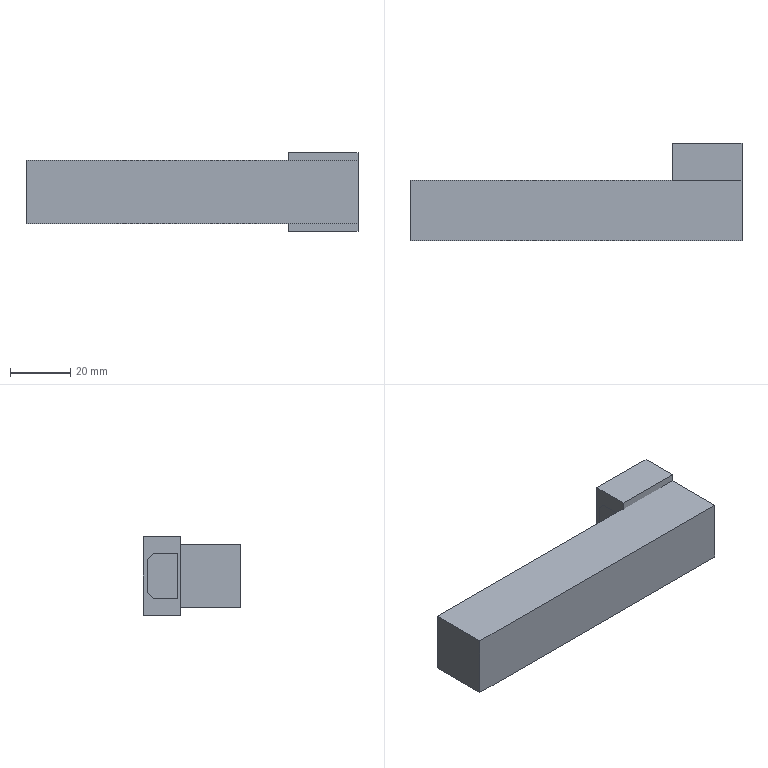Part | NX | 4 solids | 42 faces | box 110 x 32.2 x 26 mm | volume 66649 mm3 | plane 38 | cylinder 4 | commonest cylinder face diameters 6.5 x2 5.057 x1 6.503 x1
STEP:
#1=CARTESIAN_POINT('',(121.304,129.193,0.));
#2=VERTEX_POINT('',#1);
#3=CARTESIAN_POINT('',(121.304,131.193,0.));
#4=VERTEX_POINT('',#3);
#5=CARTESIAN_POINT('',(121.304,129.193,0.));
#6=DIRECTION('',(0.,1.,0.));
#7=VECTOR('',#6,1000.);
#8=LINE('',#5,#7);
#9=EDGE_CURVE('',#2,#4,#8,.T.);
#10=ORIENTED_EDGE('',*,*,#9,.T.);
#11=CARTESIAN_POINT('',(121.304,131.193,15.));
#12=VERTEX_POINT('',#11);
#13=CARTESIAN_POINT('',(121.304,131.193,15.));
#14=DIRECTION('',(0.,0.,-1.));
#15=VECTOR('',#14,1000.);
#16=LINE('',#13,#15);
#17=EDGE_CURVE('',#12,#4,#16,.T.);
#18=ORIENTED_EDGE('',*,*,#17,.F.);
#19=CARTESIAN_POINT('',(121.304,129.193,15.));
#20=VERTEX_POINT('',#19);
#21=CARTESIAN_POINT('',(121.304,129.193,15.));
#22=DIRECTION('',(0.,1.,0.));
#23=VECTOR('',#22,1000.);
#24=LINE('',#21,#23);
#25=EDGE_CURVE('',#20,#12,#24,.T.);
#26=ORIENTED_EDGE('',*,*,#25,.F.);
#27=CARTESIAN_POINT('',(121.304,129.193,15.));
#28=DIRECTION('',(0.,0.,-1.));
#29=VECTOR('',#28,1000.);
#30=LINE('',#27,#29);
#31=EDGE_CURVE('',#20,#2,#30,.T.);
#32=ORIENTED_EDGE('',*,*,#31,.T.);
#33=EDGE_LOOP('',(#10,#18,#26,#32));
#34=FACE_BOUND('',#33,.T.);
#35=CARTESIAN_POINT('',(121.304,129.193,15.));
#36=DIRECTION('',(-1.,0.,0.));
#37=DIRECTION('',(0.,0.,1.));
#38=AXIS2_PLACEMENT_3D('',#35,#36,#37);
#39=PLANE('',#38);
#40=ADVANCED_FACE('',(#34),#39,.F.);
#41=CARTESIAN_POINT('',(127.304,131.193,10.028));
#42=VERTEX_POINT('',#41);
#43=CARTESIAN_POINT('',(127.304,131.193,7.5));
#44=DIRECTION('',(0.,1.,0.));
#45=DIRECTION('',(0.,0.,1.));
#46=AXIS2_PLACEMENT_3D('',#43,#44,#45);
#47=CIRCLE('',#46,2.529);
#48=EDGE_CURVE('',#42,#42,#47,.T.);
#49=ORIENTED_EDGE('',*,*,#48,.T.);
#50=EDGE_LOOP('',(#49));
#51=FACE_BOUND('',#50,.T.);
#52=CARTESIAN_POINT('',(133.304,131.193,0.));
#53=VERTEX_POINT('',#52);
#54=CARTESIAN_POINT('',(121.304,131.193,0.));
#55=DIRECTION('',(1.,0.,0.));
#56=VECTOR('',#55,1000.);
#57=LINE('',#54,#56);
#58=EDGE_CURVE('',#4,#53,#57,.T.);
#59=ORIENTED_EDGE('',*,*,#58,.T.);
#60=CARTESIAN_POINT('',(133.304,131.193,15.));
#61=VERTEX_POINT('',#60);
#62=CARTESIAN_POINT('',(133.304,131.193,15.));
#63=DIRECTION('',(0.,0.,-1.));
#64=VECTOR('',#63,1000.);
#65=LINE('',#62,#64);
#66=EDGE_CURVE('',#61,#53,#65,.T.);
#67=ORIENTED_EDGE('',*,*,#66,.F.);
#68=CARTESIAN_POINT('',(121.304,131.193,15.));
#69=DIRECTION('',(1.,0.,0.));
#70=VECTOR('',#69,1000.);
#71=LINE('',#68,#70);
#72=EDGE_CURVE('',#12,#61,#71,.T.);
#73=ORIENTED_EDGE('',*,*,#72,.F.);
#74=ORIENTED_EDGE('',*,*,#17,.T.);
#75=EDGE_LOOP('',(#59,#67,#73,#74));
#76=FACE_BOUND('',#75,.T.);
#77=CARTESIAN_POINT('',(121.304,131.193,15.));
#78=DIRECTION('',(0.,1.,0.));
#79=DIRECTION('',(0.,0.,1.));
#80=AXIS2_PLACEMENT_3D('',#77,#78,#79);
#81=PLANE('',#80);
#82=ADVANCED_FACE('',(#51,#76),#81,.F.);
#83=CARTESIAN_POINT('',(133.304,129.193,0.));
#84=VERTEX_POINT('',#83);
#85=CARTESIAN_POINT('',(133.304,131.193,0.));
#86=DIRECTION('',(0.,-1.,0.));
#87=VECTOR('',#86,1000.);
#88=LINE('',#85,#87);
#89=EDGE_CURVE('',#53,#84,#88,.T.);
#90=ORIENTED_EDGE('',*,*,#89,.T.);
#91=CARTESIAN_POINT('',(133.304,129.193,15.));
#92=VERTEX_POINT('',#91);
#93=CARTESIAN_POINT('',(133.304,129.193,15.));
#94=DIRECTION('',(0.,0.,-1.));
#95=VECTOR('',#94,1000.);
#96=LINE('',#93,#95);
#97=EDGE_CURVE('',#92,#84,#96,.T.);
#98=ORIENTED_EDGE('',*,*,#97,.F.);
#99=CARTESIAN_POINT('',(133.304,131.193,15.));
#100=DIRECTION('',(0.,-1.,0.));
#101=VECTOR('',#100,1000.);
#102=LINE('',#99,#101);
#103=EDGE_CURVE('',#61,#92,#102,.T.);
#104=ORIENTED_EDGE('',*,*,#103,.F.);
#105=ORIENTED_EDGE('',*,*,#66,.T.);
#106=EDGE_LOOP('',(#90,#98,#104,#105));
#107=FACE_BOUND('',#106,.T.);
#108=CARTESIAN_POINT('',(133.304,131.193,15.));
#109=DIRECTION('',(1.,0.,0.));
#110=DIRECTION('',(0.,0.,-1.));
#111=AXIS2_PLACEMENT_3D('',#108,#109,#110);
#112=PLANE('',#111);
#113=ADVANCED_FACE('',(#107),#112,.F.);
#114=CARTESIAN_POINT('',(136.304,129.193,0.));
#115=VERTEX_POINT('',#114);
#116=CARTESIAN_POINT('',(133.304,129.193,0.));
#117=DIRECTION('',(1.,0.,0.));
#118=VECTOR('',#117,1000.);
#119=LINE('',#116,#118);
#120=EDGE_CURVE('',#84,#115,#119,.T.);
#121=ORIENTED_EDGE('',*,*,#120,.T.);
#122=CARTESIAN_POINT('',(136.304,129.193,15.));
#123=VERTEX_POINT('',#122);
#124=CARTESIAN_POINT('',(136.304,129.193,15.));
#125=DIRECTION('',(0.,0.,-1.));
#126=VECTOR('',#125,1000.);
#127=LINE('',#124,#126);
#128=EDGE_CURVE('',#123,#115,#127,.T.);
#129=ORIENTED_EDGE('',*,*,#128,.F.);
#130=CARTESIAN_POINT('',(133.304,129.193,15.));
#131=DIRECTION('',(1.,0.,0.));
#132=VECTOR('',#131,1000.);
#133=LINE('',#130,#132);
#134=EDGE_CURVE('',#92,#123,#133,.T.);
#135=ORIENTED_EDGE('',*,*,#134,.F.);
#136=ORIENTED_EDGE('',*,*,#97,.T.);
#137=EDGE_LOOP('',(#121,#129,#135,#136));
#138=FACE_BOUND('',#137,.T.);
#139=CARTESIAN_POINT('',(133.304,129.193,15.));
#140=DIRECTION('',(0.,1.,0.));
#141=DIRECTION('',(0.,0.,1.));
#142=AXIS2_PLACEMENT_3D('',#139,#140,#141);
#143=PLANE('',#142);
#144=ADVANCED_FACE('',(#138),#143,.F.);
#145=CARTESIAN_POINT('',(136.304,137.193,0.));
#146=VERTEX_POINT('',#145);
#147=CARTESIAN_POINT('',(136.304,137.193,0.));
#148=DIRECTION('',(0.,1.,0.));
#149=VECTOR('',#148,1000.);
#150=LINE('',#147,#149);
#151=EDGE_CURVE('',#115,#146,#150,.T.);
#152=ORIENTED_EDGE('',*,*,#151,.T.);
#153=CARTESIAN_POINT('',(136.304,139.193,2.));
#154=VERTEX_POINT('',#153);
#155=CARTESIAN_POINT('',(136.304,139.193,2.));
#156=DIRECTION('',(0.,0.7071,0.7071));
#157=VECTOR('',#156,1000.);
#158=LINE('',#155,#157);
#159=EDGE_CURVE('',#146,#154,#158,.T.);
#160=ORIENTED_EDGE('',*,*,#159,.T.);
#161=CARTESIAN_POINT('',(136.304,139.193,13.));
#162=VERTEX_POINT('',#161);
#163=CARTESIAN_POINT('',(136.304,139.193,15.));
#164=DIRECTION('',(0.,0.,-1.));
#165=VECTOR('',#164,1000.);
#166=LINE('',#163,#165);
#167=EDGE_CURVE('',#162,#154,#166,.T.);
#168=ORIENTED_EDGE('',*,*,#167,.F.);
#169=CARTESIAN_POINT('',(136.304,137.193,15.));
#170=VERTEX_POINT('',#169);
#171=CARTESIAN_POINT('',(136.304,137.193,15.));
#172=DIRECTION('',(0.,0.7071,-0.7071));
#173=VECTOR('',#172,1000.);
#174=LINE('',#171,#173);
#175=EDGE_CURVE('',#162,#170,#174,.F.);
#176=ORIENTED_EDGE('',*,*,#175,.T.);
#177=CARTESIAN_POINT('',(136.304,129.193,15.));
#178=DIRECTION('',(0.,1.,0.));
#179=VECTOR('',#178,1000.);
#180=LINE('',#177,#179);
#181=EDGE_CURVE('',#123,#170,#180,.T.);
#182=ORIENTED_EDGE('',*,*,#181,.F.);
#183=ORIENTED_EDGE('',*,*,#128,.T.);
#184=EDGE_LOOP('',(#152,#160,#168,#176,#182,#183));
#185=FACE_BOUND('',#184,.T.);
#186=CARTESIAN_POINT('',(136.304,137.193,15.));
#187=DIRECTION('',(-1.,0.,0.));
#188=DIRECTION('',(0.,0.,1.));
#189=AXIS2_PLACEMENT_3D('',#186,#187,#188);
#190=PLANE('',#189);
#191=ADVANCED_FACE('',(#185),#190,.F.);
#192=CARTESIAN_POINT('',(127.304,139.193,4.972));
#193=VERTEX_POINT('',#192);
#194=CARTESIAN_POINT('',(127.304,139.193,7.5));
#195=DIRECTION('',(0.,-1.,0.));
#196=DIRECTION('',(0.,0.,-1.));
#197=AXIS2_PLACEMENT_3D('',#194,#195,#196);
#198=CIRCLE('',#197,2.529);
#199=EDGE_CURVE('',#193,#193,#198,.T.);
#200=ORIENTED_EDGE('',*,*,#199,.T.);
#201=EDGE_LOOP('',(#200));
#202=FACE_BOUND('',#201,.T.);
#203=ORIENTED_EDGE('',*,*,#167,.T.);
#204=CARTESIAN_POINT('',(118.304,139.193,2.));
#205=VERTEX_POINT('',#204);
#206=CARTESIAN_POINT('',(118.304,139.193,2.));
#207=DIRECTION('',(-1.,0.,0.));
#208=VECTOR('',#207,1000.);
#209=LINE('',#206,#208);
#210=EDGE_CURVE('',#154,#205,#209,.T.);
#211=ORIENTED_EDGE('',*,*,#210,.T.);
#212=CARTESIAN_POINT('',(118.304,139.193,13.));
#213=VERTEX_POINT('',#212);
#214=CARTESIAN_POINT('',(118.304,139.193,15.));
#215=DIRECTION('',(0.,0.,-1.));
#216=VECTOR('',#215,1000.);
#217=LINE('',#214,#216);
#218=EDGE_CURVE('',#213,#205,#217,.T.);
#219=ORIENTED_EDGE('',*,*,#218,.F.);
#220=CARTESIAN_POINT('',(136.304,139.193,13.));
#221=DIRECTION('',(1.,0.,0.));
#222=VECTOR('',#221,1000.);
#223=LINE('',#220,#222);
#224=EDGE_CURVE('',#213,#162,#223,.T.);
#225=ORIENTED_EDGE('',*,*,#224,.T.);
#226=EDGE_LOOP('',(#203,#211,#219,#225));
#227=FACE_BOUND('',#226,.T.);
#228=CARTESIAN_POINT('',(136.304,139.193,15.));
#229=DIRECTION('',(0.,-1.,0.));
#230=DIRECTION('',(0.,0.,-1.));
#231=AXIS2_PLACEMENT_3D('',#228,#229,#230);
#232=PLANE('',#231);
#233=ADVANCED_FACE('',(#202,#227),#232,.F.);
#234=ORIENTED_EDGE('',*,*,#218,.T.);
#235=CARTESIAN_POINT('',(118.304,137.193,0.));
#236=VERTEX_POINT('',#235);
#237=CARTESIAN_POINT('',(118.304,139.193,2.));
#238=DIRECTION('',(0.,-0.7071,-0.7071));
#239=VECTOR('',#238,1000.);
#240=LINE('',#237,#239);
#241=EDGE_CURVE('',#205,#236,#240,.T.);
#242=ORIENTED_EDGE('',*,*,#241,.T.);
#243=CARTESIAN_POINT('',(118.304,129.193,0.));
#244=VERTEX_POINT('',#243);
#245=CARTESIAN_POINT('',(118.304,137.193,0.));
#246=DIRECTION('',(0.,-1.,0.));
#247=VECTOR('',#246,1000.);
#248=LINE('',#245,#247);
#249=EDGE_CURVE('',#236,#244,#248,.T.);
#250=ORIENTED_EDGE('',*,*,#249,.T.);
#251=CARTESIAN_POINT('',(118.304,129.193,15.));
#252=VERTEX_POINT('',#251);
#253=CARTESIAN_POINT('',(118.304,129.193,15.));
#254=DIRECTION('',(0.,0.,-1.));
#255=VECTOR('',#254,1000.);
#256=LINE('',#253,#255);
#257=EDGE_CURVE('',#252,#244,#256,.T.);
#258=ORIENTED_EDGE('',*,*,#257,.F.);
#259=CARTESIAN_POINT('',(118.304,137.193,15.));
#260=VERTEX_POINT('',#259);
#261=CARTESIAN_POINT('',(118.304,139.193,15.));
#262=DIRECTION('',(0.,-1.,0.));
#263=VECTOR('',#262,1000.);
#264=LINE('',#261,#263);
#265=EDGE_CURVE('',#260,#252,#264,.T.);
#266=ORIENTED_EDGE('',*,*,#265,.F.);
#267=CARTESIAN_POINT('',(118.304,137.193,15.));
#268=DIRECTION('',(0.,-0.7071,0.7071));
#269=VECTOR('',#268,1000.);
#270=LINE('',#267,#269);
#271=EDGE_CURVE('',#260,#213,#270,.F.);
#272=ORIENTED_EDGE('',*,*,#271,.T.);
#273=EDGE_LOOP('',(#234,#242,#250,#258,#266,#272));
#274=FACE_BOUND('',#273,.T.);
#275=CARTESIAN_POINT('',(118.304,137.193,15.));
#276=DIRECTION('',(1.,0.,0.));
#277=DIRECTION('',(0.,0.,-1.));
#278=AXIS2_PLACEMENT_3D('',#275,#276,#277);
#279=PLANE('',#278);
#280=ADVANCED_FACE('',(#274),#279,.F.);
#281=CARTESIAN_POINT('',(118.304,129.193,0.));
#282=DIRECTION('',(1.,0.,0.));
#283=VECTOR('',#282,1000.);
#284=LINE('',#281,#283);
#285=EDGE_CURVE('',#244,#2,#284,.T.);
#286=ORIENTED_EDGE('',*,*,#285,.T.);
#287=ORIENTED_EDGE('',*,*,#31,.F.);
#288=CARTESIAN_POINT('',(118.304,129.193,15.));
#289=DIRECTION('',(1.,0.,0.));
#290=VECTOR('',#289,1000.);
#291=LINE('',#288,#290);
#292=EDGE_CURVE('',#252,#20,#291,.T.);
#293=ORIENTED_EDGE('',*,*,#292,.F.);
#294=ORIENTED_EDGE('',*,*,#257,.T.);
#295=EDGE_LOOP('',(#286,#287,#293,#294));
#296=FACE_BOUND('',#295,.T.);
#297=CARTESIAN_POINT('',(118.304,129.193,15.));
#298=DIRECTION('',(0.,1.,0.));
#299=DIRECTION('',(0.,0.,1.));
#300=AXIS2_PLACEMENT_3D('',#297,#298,#299);
#301=PLANE('',#300);
#302=ADVANCED_FACE('',(#296),#301,.F.);
#303=ORIENTED_EDGE('',*,*,#181,.T.);
#304=CARTESIAN_POINT('',(0.,137.193,15.));
#305=DIRECTION('',(-1.,0.,0.));
#306=VECTOR('',#305,1000.);
#307=LINE('',#304,#306);
#308=EDGE_CURVE('',#170,#260,#307,.T.);
#309=ORIENTED_EDGE('',*,*,#308,.T.);
#310=ORIENTED_EDGE('',*,*,#265,.T.);
#311=ORIENTED_EDGE('',*,*,#292,.T.);
#312=ORIENTED_EDGE('',*,*,#25,.T.);
#313=ORIENTED_EDGE('',*,*,#72,.T.);
#314=ORIENTED_EDGE('',*,*,#103,.T.);
#315=ORIENTED_EDGE('',*,*,#134,.T.);
#316=EDGE_LOOP('',(#303,#309,#310,#311,#312,#313,#314,#315));
#317=FACE_BOUND('',#316,.T.);
#318=CARTESIAN_POINT('',(0.,0.,15.));
#319=DIRECTION('',(0.,0.,-1.));
#320=DIRECTION('',(-1.,0.,0.));
#321=AXIS2_PLACEMENT_3D('',#318,#319,#320);
#322=PLANE('',#321);
#323=ADVANCED_FACE('',(#317),#322,.F.);
#324=ORIENTED_EDGE('',*,*,#249,.F.);
#325=CARTESIAN_POINT('',(136.304,137.193,0.));
#326=DIRECTION('',(1.,0.,0.));
#327=VECTOR('',#326,1000.);
#328=LINE('',#325,#327);
#329=EDGE_CURVE('',#236,#146,#328,.T.);
#330=ORIENTED_EDGE('',*,*,#329,.T.);
#331=ORIENTED_EDGE('',*,*,#151,.F.);
#332=ORIENTED_EDGE('',*,*,#120,.F.);
#333=ORIENTED_EDGE('',*,*,#89,.F.);
#334=ORIENTED_EDGE('',*,*,#58,.F.);
#335=ORIENTED_EDGE('',*,*,#9,.F.);
#336=ORIENTED_EDGE('',*,*,#285,.F.);
#337=EDGE_LOOP('',(#324,#330,#331,#332,#333,#334,#335,#336));
#338=FACE_BOUND('',#337,.T.);
#339=CARTESIAN_POINT('',(0.,0.,0.));
#340=DIRECTION('',(0.,0.,-1.));
#341=DIRECTION('',(-1.,0.,0.));
#342=AXIS2_PLACEMENT_3D('',#339,#340,#341);
#343=PLANE('',#342);
#344=ADVANCED_FACE('',(#338),#343,.T.);
#345=ORIENTED_EDGE('',*,*,#159,.F.);
#346=ORIENTED_EDGE('',*,*,#329,.F.);
#347=ORIENTED_EDGE('',*,*,#241,.F.);
#348=ORIENTED_EDGE('',*,*,#210,.F.);
#349=EDGE_LOOP('',(#345,#346,#347,#348));
#350=FACE_BOUND('',#349,.T.);
#351=CARTESIAN_POINT('',(136.304,139.193,2.));
#352=DIRECTION('',(0.,0.7071,-0.7071));
#353=DIRECTION('',(1.,0.,0.));
#354=AXIS2_PLACEMENT_3D('',#351,#352,#353);
#355=PLANE('',#354);
#356=ADVANCED_FACE('',(#350),#355,.T.);
#357=ORIENTED_EDGE('',*,*,#175,.F.);
#358=ORIENTED_EDGE('',*,*,#224,.F.);
#359=ORIENTED_EDGE('',*,*,#271,.F.);
#360=ORIENTED_EDGE('',*,*,#308,.F.);
#361=EDGE_LOOP('',(#357,#358,#359,#360));
#362=FACE_BOUND('',#361,.T.);
#363=CARTESIAN_POINT('',(0.,137.193,15.));
#364=DIRECTION('',(0.,-0.7071,-0.7071));
#365=DIRECTION('',(-1.,0.,0.));
#366=AXIS2_PLACEMENT_3D('',#363,#364,#365);
#367=PLANE('',#366);
#368=ADVANCED_FACE('',(#362),#367,.F.);
#369=ORIENTED_EDGE('',*,*,#199,.F.);
#370=EDGE_LOOP('',(#369));
#371=FACE_BOUND('',#370,.T.);
#372=ORIENTED_EDGE('',*,*,#48,.F.);
#373=EDGE_LOOP('',(#372));
#374=FACE_BOUND('',#373,.T.);
#375=CARTESIAN_POINT('',(127.304,141.693,7.5));
#376=DIRECTION('',(0.,-1.,0.));
#377=DIRECTION('',(0.,0.,-1.));
#378=AXIS2_PLACEMENT_3D('',#375,#376,#377);
#379=CYLINDRICAL_SURFACE('',#378,2.529);
#380=ADVANCED_FACE('',(#371,#374),#379,.F.);
#381=CLOSED_SHELL('',(#40,#82,#113,#144,#191,#233,#280,#302,#323,#344,#356,#368,#380));
#382=MANIFOLD_SOLID_BREP('',#381);
#383=CARTESIAN_POINT('',(141.304,108.193,18.));
#384=VERTEX_POINT('',#383);
#385=CARTESIAN_POINT('',(31.304,108.193,18.));
#386=VERTEX_POINT('',#385);
#387=CARTESIAN_POINT('',(86.304,108.193,18.));
#388=DIRECTION('',(-1.,0.,0.));
#389=VECTOR('',#388,1000.);
#390=LINE('',#387,#389);
#391=EDGE_CURVE('',#384,#386,#390,.T.);
#392=ORIENTED_EDGE('',*,*,#391,.F.);
#393=CARTESIAN_POINT('',(141.304,128.193,18.));
#394=VERTEX_POINT('',#393);
#395=CARTESIAN_POINT('',(141.304,120.693,18.));
#396=DIRECTION('',(0.,-1.,0.));
#397=VECTOR('',#396,1000.);
#398=LINE('',#395,#397);
#399=EDGE_CURVE('',#394,#384,#398,.T.);
#400=ORIENTED_EDGE('',*,*,#399,.F.);
#401=CARTESIAN_POINT('',(31.304,128.193,18.));
#402=VERTEX_POINT('',#401);
#403=CARTESIAN_POINT('',(86.304,128.193,18.));
#404=DIRECTION('',(1.,0.,0.));
#405=VECTOR('',#404,1000.);
#406=LINE('',#403,#405);
#407=EDGE_CURVE('',#402,#394,#406,.T.);
#408=ORIENTED_EDGE('',*,*,#407,.F.);
#409=CARTESIAN_POINT('',(31.304,120.693,18.));
#410=DIRECTION('',(0.,1.,0.));
#411=VECTOR('',#410,1000.);
#412=LINE('',#409,#411);
#413=EDGE_CURVE('',#386,#402,#412,.T.);
#414=ORIENTED_EDGE('',*,*,#413,.F.);
#415=EDGE_LOOP('',(#392,#400,#408,#414));
#416=FACE_BOUND('',#415,.T.);
#417=CARTESIAN_POINT('',(86.304,120.693,18.));
#418=DIRECTION('',(0.,0.,1.));
#419=DIRECTION('',(1.,0.,0.));
#420=AXIS2_PLACEMENT_3D('',#417,#418,#419);
#421=PLANE('',#420);
#422=ADVANCED_FACE('',(#416),#421,.T.);
#423=CARTESIAN_POINT('',(141.304,108.193,-3.));
#424=VERTEX_POINT('',#423);
#425=CARTESIAN_POINT('',(141.304,108.193,0.));
#426=DIRECTION('',(0.,0.,1.));
#427=VECTOR('',#426,1000.);
#428=LINE('',#425,#427);
#429=EDGE_CURVE('',#424,#384,#428,.T.);
#430=ORIENTED_EDGE('',*,*,#429,.T.);
#431=ORIENTED_EDGE('',*,*,#391,.T.);
#432=CARTESIAN_POINT('',(31.304,108.193,-3.));
#433=VERTEX_POINT('',#432);
#434=CARTESIAN_POINT('',(31.304,108.193,0.));
#435=DIRECTION('',(0.,0.,1.));
#436=VECTOR('',#435,1000.);
#437=LINE('',#434,#436);
#438=EDGE_CURVE('',#433,#386,#437,.T.);
#439=ORIENTED_EDGE('',*,*,#438,.F.);
#440=CARTESIAN_POINT('',(86.304,108.193,-3.));
#441=DIRECTION('',(1.,0.,0.));
#442=VECTOR('',#441,1000.);
#443=LINE('',#440,#442);
#444=EDGE_CURVE('',#433,#424,#443,.T.);
#445=ORIENTED_EDGE('',*,*,#444,.T.);
#446=EDGE_LOOP('',(#430,#431,#439,#445));
#447=FACE_BOUND('',#446,.T.);
#448=CARTESIAN_POINT('',(86.304,108.193,0.));
#449=DIRECTION('',(0.,-1.,0.));
#450=DIRECTION('',(0.,0.,-1.));
#451=AXIS2_PLACEMENT_3D('',#448,#449,#450);
#452=PLANE('',#451);
#453=ADVANCED_FACE('',(#447),#452,.T.);
#454=ORIENTED_EDGE('',*,*,#438,.T.);
#455=ORIENTED_EDGE('',*,*,#413,.T.);
#456=CARTESIAN_POINT('',(31.304,128.193,-3.));
#457=VERTEX_POINT('',#456);
#458=CARTESIAN_POINT('',(31.304,128.193,0.));
#459=DIRECTION('',(0.,0.,1.));
#460=VECTOR('',#459,1000.);
#461=LINE('',#458,#460);
#462=EDGE_CURVE('',#457,#402,#461,.T.);
#463=ORIENTED_EDGE('',*,*,#462,.F.);
#464=CARTESIAN_POINT('',(31.304,120.693,-3.));
#465=DIRECTION('',(0.,-1.,0.));
#466=VECTOR('',#465,1000.);
#467=LINE('',#464,#466);
#468=EDGE_CURVE('',#457,#433,#467,.T.);
#469=ORIENTED_EDGE('',*,*,#468,.T.);
#470=EDGE_LOOP('',(#454,#455,#463,#469));
#471=FACE_BOUND('',#470,.T.);
#472=CARTESIAN_POINT('',(31.304,120.693,0.));
#473=DIRECTION('',(-1.,0.,0.));
#474=DIRECTION('',(0.,0.,1.));
#475=AXIS2_PLACEMENT_3D('',#472,#473,#474);
#476=PLANE('',#475);
#477=ADVANCED_FACE('',(#471),#476,.T.);
#478=ORIENTED_EDGE('',*,*,#462,.T.);
#479=ORIENTED_EDGE('',*,*,#407,.T.);
#480=CARTESIAN_POINT('',(141.304,128.193,-3.));
#481=VERTEX_POINT('',#480);
#482=CARTESIAN_POINT('',(141.304,128.193,0.));
#483=DIRECTION('',(0.,0.,1.));
#484=VECTOR('',#483,1000.);
#485=LINE('',#482,#484);
#486=EDGE_CURVE('',#481,#394,#485,.T.);
#487=ORIENTED_EDGE('',*,*,#486,.F.);
#488=CARTESIAN_POINT('',(86.304,128.193,-3.));
#489=DIRECTION('',(-1.,0.,0.));
#490=VECTOR('',#489,1000.);
#491=LINE('',#488,#490);
#492=EDGE_CURVE('',#481,#457,#491,.T.);
#493=ORIENTED_EDGE('',*,*,#492,.T.);
#494=EDGE_LOOP('',(#478,#479,#487,#493));
#495=FACE_BOUND('',#494,.T.);
#496=CARTESIAN_POINT('',(86.304,128.193,0.));
#497=DIRECTION('',(0.,1.,0.));
#498=DIRECTION('',(0.,0.,1.));
#499=AXIS2_PLACEMENT_3D('',#496,#497,#498);
#500=PLANE('',#499);
#501=ADVANCED_FACE('',(#495),#500,.T.);
#502=CARTESIAN_POINT('',(141.304,120.693,-3.));
#503=DIRECTION('',(0.,1.,0.));
#504=VECTOR('',#503,1000.);
#505=LINE('',#502,#504);
#506=EDGE_CURVE('',#424,#481,#505,.T.);
#507=ORIENTED_EDGE('',*,*,#506,.F.);
#508=ORIENTED_EDGE('',*,*,#444,.F.);
#509=ORIENTED_EDGE('',*,*,#468,.F.);
#510=ORIENTED_EDGE('',*,*,#492,.F.);
#511=EDGE_LOOP('',(#507,#508,#509,#510));
#512=FACE_BOUND('',#511,.T.);
#513=CARTESIAN_POINT('',(86.304,120.693,-3.));
#514=DIRECTION('',(0.,0.,-1.));
#515=DIRECTION('',(-1.,0.,0.));
#516=AXIS2_PLACEMENT_3D('',#513,#514,#515);
#517=PLANE('',#516);
#518=ADVANCED_FACE('',(#512),#517,.T.);
#519=ORIENTED_EDGE('',*,*,#506,.T.);
#520=ORIENTED_EDGE('',*,*,#486,.T.);
#521=ORIENTED_EDGE('',*,*,#399,.T.);
#522=ORIENTED_EDGE('',*,*,#429,.F.);
#523=EDGE_LOOP('',(#519,#520,#521,#522));
#524=FACE_BOUND('',#523,.T.);
#525=CARTESIAN_POINT('',(141.304,120.693,0.));
#526=DIRECTION('',(1.,0.,0.));
#527=DIRECTION('',(0.,0.,-1.));
#528=AXIS2_PLACEMENT_3D('',#525,#526,#527);
#529=PLANE('',#528);
#530=ADVANCED_FACE('',(#524),#529,.T.);
#531=CLOSED_SHELL('',(#422,#453,#477,#501,#518,#530));
#532=MANIFOLD_SOLID_BREP('',#531);
#533=CARTESIAN_POINT('',(141.304,127.993,20.5));
#534=VERTEX_POINT('',#533);
#535=CARTESIAN_POINT('',(118.304,127.993,20.5));
#536=VERTEX_POINT('',#535);
#537=CARTESIAN_POINT('',(127.304,127.993,20.5));
#538=DIRECTION('',(-1.,0.,0.));
#539=VECTOR('',#538,1000.);
#540=LINE('',#537,#539);
#541=EDGE_CURVE('',#534,#536,#540,.T.);
#542=ORIENTED_EDGE('',*,*,#541,.F.);
#543=CARTESIAN_POINT('',(141.304,140.393,20.5));
#544=VERTEX_POINT('',#543);
#545=CARTESIAN_POINT('',(141.304,134.193,20.5));
#546=DIRECTION('',(0.,-1.,0.));
#547=VECTOR('',#546,1000.);
#548=LINE('',#545,#547);
#549=EDGE_CURVE('',#544,#534,#548,.T.);
#550=ORIENTED_EDGE('',*,*,#549,.F.);
#551=CARTESIAN_POINT('',(118.304,140.393,20.5));
#552=VERTEX_POINT('',#551);
#553=CARTESIAN_POINT('',(127.304,140.393,20.5));
#554=DIRECTION('',(1.,0.,0.));
#555=VECTOR('',#554,1000.);
#556=LINE('',#553,#555);
#557=EDGE_CURVE('',#552,#544,#556,.T.);
#558=ORIENTED_EDGE('',*,*,#557,.F.);
#559=CARTESIAN_POINT('',(118.304,134.193,20.5));
#560=DIRECTION('',(0.,1.,0.));
#561=VECTOR('',#560,1000.);
#562=LINE('',#559,#561);
#563=EDGE_CURVE('',#536,#552,#562,.T.);
#564=ORIENTED_EDGE('',*,*,#563,.F.);
#565=EDGE_LOOP('',(#542,#550,#558,#564));
#566=FACE_BOUND('',#565,.T.);
#567=CARTESIAN_POINT('',(127.304,134.193,20.5));
#568=DIRECTION('',(0.,0.,1.));
#569=DIRECTION('',(1.,0.,0.));
#570=AXIS2_PLACEMENT_3D('',#567,#568,#569);
#571=PLANE('',#570);
#572=ADVANCED_FACE('',(#566),#571,.T.);
#573=CARTESIAN_POINT('',(141.304,127.993,-5.5));
#574=VERTEX_POINT('',#573);
#575=CARTESIAN_POINT('',(141.304,127.993,0.));
#576=DIRECTION('',(0.,0.,1.));
#577=VECTOR('',#576,1000.);
#578=LINE('',#575,#577);
#579=EDGE_CURVE('',#574,#534,#578,.T.);
#580=ORIENTED_EDGE('',*,*,#579,.T.);
#581=ORIENTED_EDGE('',*,*,#541,.T.);
#582=CARTESIAN_POINT('',(118.304,127.993,-5.5));
#583=VERTEX_POINT('',#582);
#584=CARTESIAN_POINT('',(118.304,127.993,0.));
#585=DIRECTION('',(0.,0.,1.));
#586=VECTOR('',#585,1000.);
#587=LINE('',#584,#586);
#588=EDGE_CURVE('',#583,#536,#587,.T.);
#589=ORIENTED_EDGE('',*,*,#588,.F.);
#590=CARTESIAN_POINT('',(127.304,127.993,-5.5));
#591=DIRECTION('',(1.,0.,0.));
#592=VECTOR('',#591,1000.);
#593=LINE('',#590,#592);
#594=EDGE_CURVE('',#583,#574,#593,.T.);
#595=ORIENTED_EDGE('',*,*,#594,.T.);
#596=EDGE_LOOP('',(#580,#581,#589,#595));
#597=FACE_BOUND('',#596,.T.);
#598=CARTESIAN_POINT('',(127.304,127.993,0.));
#599=DIRECTION('',(0.,-1.,0.));
#600=DIRECTION('',(0.,0.,-1.));
#601=AXIS2_PLACEMENT_3D('',#598,#599,#600);
#602=PLANE('',#601);
#603=ADVANCED_FACE('',(#597),#602,.T.);
#604=ORIENTED_EDGE('',*,*,#588,.T.);
#605=ORIENTED_EDGE('',*,*,#563,.T.);
#606=CARTESIAN_POINT('',(118.304,140.393,-5.5));
#607=VERTEX_POINT('',#606);
#608=CARTESIAN_POINT('',(118.304,140.393,0.));
#609=DIRECTION('',(0.,0.,1.));
#610=VECTOR('',#609,1000.);
#611=LINE('',#608,#610);
#612=EDGE_CURVE('',#607,#552,#611,.T.);
#613=ORIENTED_EDGE('',*,*,#612,.F.);
#614=CARTESIAN_POINT('',(118.304,134.193,-5.5));
#615=DIRECTION('',(0.,-1.,0.));
#616=VECTOR('',#615,1000.);
#617=LINE('',#614,#616);
#618=EDGE_CURVE('',#607,#583,#617,.T.);
#619=ORIENTED_EDGE('',*,*,#618,.T.);
#620=EDGE_LOOP('',(#604,#605,#613,#619));
#621=FACE_BOUND('',#620,.T.);
#622=CARTESIAN_POINT('',(118.304,134.193,0.));
#623=DIRECTION('',(-1.,0.,0.));
#624=DIRECTION('',(0.,0.,1.));
#625=AXIS2_PLACEMENT_3D('',#622,#623,#624);
#626=PLANE('',#625);
#627=ADVANCED_FACE('',(#621),#626,.T.);
#628=ORIENTED_EDGE('',*,*,#612,.T.);
#629=ORIENTED_EDGE('',*,*,#557,.T.);
#630=CARTESIAN_POINT('',(141.304,140.393,-5.5));
#631=VERTEX_POINT('',#630);
#632=CARTESIAN_POINT('',(141.304,140.393,0.));
#633=DIRECTION('',(0.,0.,1.));
#634=VECTOR('',#633,1000.);
#635=LINE('',#632,#634);
#636=EDGE_CURVE('',#631,#544,#635,.T.);
#637=ORIENTED_EDGE('',*,*,#636,.F.);
#638=CARTESIAN_POINT('',(127.304,140.393,-5.5));
#639=DIRECTION('',(-1.,0.,0.));
#640=VECTOR('',#639,1000.);
#641=LINE('',#638,#640);
#642=EDGE_CURVE('',#631,#607,#641,.T.);
#643=ORIENTED_EDGE('',*,*,#642,.T.);
#644=EDGE_LOOP('',(#628,#629,#637,#643));
#645=FACE_BOUND('',#644,.T.);
#646=CARTESIAN_POINT('',(127.304,140.393,0.));
#647=DIRECTION('',(0.,1.,0.));
#648=DIRECTION('',(0.,0.,1.));
#649=AXIS2_PLACEMENT_3D('',#646,#647,#648);
#650=PLANE('',#649);
#651=ADVANCED_FACE('',(#645),#650,.T.);
#652=CARTESIAN_POINT('',(141.304,134.193,-5.5));
#653=DIRECTION('',(0.,1.,0.));
#654=VECTOR('',#653,1000.);
#655=LINE('',#652,#654);
#656=EDGE_CURVE('',#574,#631,#655,.T.);
#657=ORIENTED_EDGE('',*,*,#656,.F.);
#658=ORIENTED_EDGE('',*,*,#594,.F.);
#659=ORIENTED_EDGE('',*,*,#618,.F.);
#660=ORIENTED_EDGE('',*,*,#642,.F.);
#661=EDGE_LOOP('',(#657,#658,#659,#660));
#662=FACE_BOUND('',#661,.T.);
#663=CARTESIAN_POINT('',(127.304,134.193,-5.5));
#664=DIRECTION('',(0.,0.,-1.));
#665=DIRECTION('',(-1.,0.,0.));
#666=AXIS2_PLACEMENT_3D('',#663,#664,#665);
#667=PLANE('',#666);
#668=ADVANCED_FACE('',(#662),#667,.T.);
#669=ORIENTED_EDGE('',*,*,#656,.T.);
#670=ORIENTED_EDGE('',*,*,#636,.T.);
#671=ORIENTED_EDGE('',*,*,#549,.T.);
#672=ORIENTED_EDGE('',*,*,#579,.F.);
#673=EDGE_LOOP('',(#669,#670,#671,#672));
#674=FACE_BOUND('',#673,.T.);
#675=CARTESIAN_POINT('',(141.304,134.193,0.));
#676=DIRECTION('',(1.,0.,0.));
#677=DIRECTION('',(0.,0.,-1.));
#678=AXIS2_PLACEMENT_3D('',#675,#676,#677);
#679=PLANE('',#678);
#680=ADVANCED_FACE('',(#674),#679,.T.);
#681=CLOSED_SHELL('',(#572,#603,#627,#651,#668,#680));
#682=MANIFOLD_SOLID_BREP('',#681);
#683=CARTESIAN_POINT('',(43.304,128.193,4.25));
#684=VERTEX_POINT('',#683);
#685=CARTESIAN_POINT('',(43.304,128.193,10.75));
#686=VERTEX_POINT('',#685);
#687=CARTESIAN_POINT('',(43.304,128.193,7.5));
#688=DIRECTION('',(0.,1.,0.));
#689=DIRECTION('',(1.,0.,0.));
#690=AXIS2_PLACEMENT_3D('',#687,#688,#689);
#691=CIRCLE('',#690,3.25);
#692=EDGE_CURVE('',#684,#686,#691,.T.);
#693=ORIENTED_EDGE('',*,*,#692,.F.);
#694=CARTESIAN_POINT('',(108.304,128.193,4.25));
#695=VERTEX_POINT('',#694);
#696=CARTESIAN_POINT('',(108.304,128.193,4.25));
#697=DIRECTION('',(-1.,0.,0.));
#698=VECTOR('',#697,1000.);
#699=LINE('',#696,#698);
#700=EDGE_CURVE('',#695,#684,#699,.T.);
#701=ORIENTED_EDGE('',*,*,#700,.F.);
#702=CARTESIAN_POINT('',(108.304,128.193,10.75));
#703=VERTEX_POINT('',#702);
#704=CARTESIAN_POINT('',(108.304,128.193,7.5));
#705=DIRECTION('',(0.,1.,0.));
#706=DIRECTION('',(1.,0.,0.));
#707=AXIS2_PLACEMENT_3D('',#704,#705,#706);
#708=CIRCLE('',#707,3.25);
#709=EDGE_CURVE('',#703,#695,#708,.T.);
#710=ORIENTED_EDGE('',*,*,#709,.F.);
#711=CARTESIAN_POINT('',(43.304,128.193,10.75));
#712=DIRECTION('',(1.,0.,0.));
#713=VECTOR('',#712,1000.);
#714=LINE('',#711,#713);
#715=EDGE_CURVE('',#686,#703,#714,.T.);
#716=ORIENTED_EDGE('',*,*,#715,.F.);
#717=EDGE_LOOP('',(#693,#701,#710,#716));
#718=FACE_BOUND('',#717,.T.);
#719=CARTESIAN_POINT('',(38.244,128.193,14.94));
#720=VERTEX_POINT('',#719);
#721=CARTESIAN_POINT('',(121.304,128.193,14.94));
#722=VERTEX_POINT('',#721);
#723=CARTESIAN_POINT('',(43.304,128.193,14.94));
#724=DIRECTION('',(1.,0.,0.));
#725=VECTOR('',#724,1000.);
#726=LINE('',#723,#725);
#727=EDGE_CURVE('',#720,#722,#726,.T.);
#728=ORIENTED_EDGE('',*,*,#727,.T.);
#729=CARTESIAN_POINT('',(121.304,128.193,0.06));
#730=VERTEX_POINT('',#729);
#731=CARTESIAN_POINT('',(121.304,128.193,15.));
#732=DIRECTION('',(0.,0.,-1.));
#733=VECTOR('',#732,1000.);
#734=LINE('',#731,#733);
#735=EDGE_CURVE('',#722,#730,#734,.T.);
#736=ORIENTED_EDGE('',*,*,#735,.T.);
#737=CARTESIAN_POINT('',(38.244,128.193,0.06));
#738=VERTEX_POINT('',#737);
#739=CARTESIAN_POINT('',(43.304,128.193,0.06));
#740=DIRECTION('',(-1.,0.,0.));
#741=VECTOR('',#740,1000.);
#742=LINE('',#739,#741);
#743=EDGE_CURVE('',#730,#738,#742,.T.);
#744=ORIENTED_EDGE('',*,*,#743,.T.);
#745=CARTESIAN_POINT('',(36.304,128.193,2.));
#746=VERTEX_POINT('',#745);
#747=CARTESIAN_POINT('',(38.304,128.193,0.));
#748=DIRECTION('',(-0.7071,0.,0.7071));
#749=VECTOR('',#748,1000.);
#750=LINE('',#747,#749);
#751=EDGE_CURVE('',#738,#746,#750,.T.);
#752=ORIENTED_EDGE('',*,*,#751,.T.);
#753=CARTESIAN_POINT('',(36.304,128.193,13.));
#754=VERTEX_POINT('',#753);
#755=CARTESIAN_POINT('',(36.304,128.193,2.));
#756=DIRECTION('',(0.,0.,1.));
#757=VECTOR('',#756,1000.);
#758=LINE('',#755,#757);
#759=EDGE_CURVE('',#746,#754,#758,.T.);
#760=ORIENTED_EDGE('',*,*,#759,.T.);
#761=CARTESIAN_POINT('',(36.304,128.193,13.));
#762=DIRECTION('',(0.7071,0.,0.7071));
#763=VECTOR('',#762,1000.);
#764=LINE('',#761,#763);
#765=EDGE_CURVE('',#754,#720,#764,.T.);
#766=ORIENTED_EDGE('',*,*,#765,.T.);
#767=EDGE_LOOP('',(#728,#736,#744,#752,#760,#766));
#768=FACE_BOUND('',#767,.T.);
#769=CARTESIAN_POINT('',(43.304,128.193,7.5));
#770=DIRECTION('',(0.,1.,0.));
#771=DIRECTION('',(0.,0.,1.));
#772=AXIS2_PLACEMENT_3D('',#769,#770,#771);
#773=PLANE('',#772);
#774=ADVANCED_FACE('',(#718,#768),#773,.T.);
#775=ORIENTED_EDGE('',*,*,#743,.F.);
#776=CARTESIAN_POINT('',(121.304,121.193,0.06));
#777=VERTEX_POINT('',#776);
#778=CARTESIAN_POINT('',(121.304,113.193,0.06));
#779=DIRECTION('',(0.,-1.,0.));
#780=VECTOR('',#779,1000.);
#781=LINE('',#778,#780);
#782=EDGE_CURVE('',#730,#777,#781,.T.);
#783=ORIENTED_EDGE('',*,*,#782,.T.);
#784=CARTESIAN_POINT('',(133.304,121.193,0.06));
#785=VERTEX_POINT('',#784);
#786=CARTESIAN_POINT('',(118.304,121.193,0.06));
#787=DIRECTION('',(1.,0.,0.));
#788=VECTOR('',#787,1000.);
#789=LINE('',#786,#788);
#790=EDGE_CURVE('',#777,#785,#789,.T.);
#791=ORIENTED_EDGE('',*,*,#790,.T.);
#792=CARTESIAN_POINT('',(133.304,128.193,0.06));
#793=VERTEX_POINT('',#792);
#794=CARTESIAN_POINT('',(133.304,113.193,0.06));
#795=DIRECTION('',(0.,1.,0.));
#796=VECTOR('',#795,1000.);
#797=LINE('',#794,#796);
#798=EDGE_CURVE('',#785,#793,#797,.T.);
#799=ORIENTED_EDGE('',*,*,#798,.T.);
#800=CARTESIAN_POINT('',(136.304,128.193,0.06));
#801=VERTEX_POINT('',#800);
#802=CARTESIAN_POINT('',(43.304,128.193,0.06));
#803=DIRECTION('',(-1.,0.,0.));
#804=VECTOR('',#803,1000.);
#805=LINE('',#802,#804);
#806=EDGE_CURVE('',#801,#793,#805,.T.);
#807=ORIENTED_EDGE('',*,*,#806,.F.);
#808=CARTESIAN_POINT('',(136.304,116.193,0.06));
#809=VERTEX_POINT('',#808);
#810=CARTESIAN_POINT('',(136.304,113.193,0.06));
#811=DIRECTION('',(0.,1.,0.));
#812=VECTOR('',#811,1000.);
#813=LINE('',#810,#812);
#814=EDGE_CURVE('',#809,#801,#813,.T.);
#815=ORIENTED_EDGE('',*,*,#814,.F.);
#816=CARTESIAN_POINT('',(38.244,116.193,0.06));
#817=VERTEX_POINT('',#816);
#818=CARTESIAN_POINT('',(43.304,116.193,0.06));
#819=DIRECTION('',(-1.,0.,0.));
#820=VECTOR('',#819,1000.);
#821=LINE('',#818,#820);
#822=EDGE_CURVE('',#809,#817,#821,.T.);
#823=ORIENTED_EDGE('',*,*,#822,.T.);
#824=CARTESIAN_POINT('',(38.244,113.193,0.06));
#825=DIRECTION('',(0.,1.,0.));
#826=VECTOR('',#825,1000.);
#827=LINE('',#824,#826);
#828=EDGE_CURVE('',#817,#738,#827,.T.);
#829=ORIENTED_EDGE('',*,*,#828,.T.);
#830=EDGE_LOOP('',(#775,#783,#791,#799,#807,#815,#823,#829));
#831=FACE_BOUND('',#830,.T.);
#832=CARTESIAN_POINT('',(118.304,113.193,0.06));
#833=DIRECTION('',(0.,0.,-1.));
#834=DIRECTION('',(-1.,0.,0.));
#835=AXIS2_PLACEMENT_3D('',#832,#833,#834);
#836=PLANE('',#835);
#837=ADVANCED_FACE('',(#831),#836,.T.);
#838=CARTESIAN_POINT('',(127.304,116.193,10.752));
#839=VERTEX_POINT('',#838);
#840=CARTESIAN_POINT('',(127.304,116.193,7.5));
#841=DIRECTION('',(0.,1.,0.));
#842=DIRECTION('',(0.,0.,1.));
#843=AXIS2_PLACEMENT_3D('',#840,#841,#842);
#844=CIRCLE('',#843,3.252);
#845=EDGE_CURVE('',#839,#839,#844,.T.);
#846=ORIENTED_EDGE('',*,*,#845,.F.);
#847=EDGE_LOOP('',(#846));
#848=FACE_BOUND('',#847,.T.);
#849=CARTESIAN_POINT('',(127.304,121.193,10.752));
#850=VERTEX_POINT('',#849);
#851=CARTESIAN_POINT('',(127.304,121.193,7.5));
#852=DIRECTION('',(0.,1.,0.));
#853=DIRECTION('',(0.,0.,1.));
#854=AXIS2_PLACEMENT_3D('',#851,#852,#853);
#855=CIRCLE('',#854,3.252);
#856=EDGE_CURVE('',#850,#850,#855,.F.);
#857=ORIENTED_EDGE('',*,*,#856,.F.);
#858=EDGE_LOOP('',(#857));
#859=FACE_BOUND('',#858,.T.);
#860=CARTESIAN_POINT('',(127.304,113.193,7.5));
#861=DIRECTION('',(0.,1.,0.));
#862=DIRECTION('',(0.,0.,1.));
#863=AXIS2_PLACEMENT_3D('',#860,#861,#862);
#864=CYLINDRICAL_SURFACE('',#863,3.252);
#865=ADVANCED_FACE('',(#848,#859),#864,.F.);
#866=ORIENTED_EDGE('',*,*,#692,.T.);
#867=CARTESIAN_POINT('',(43.304,116.193,10.75));
#868=VERTEX_POINT('',#867);
#869=CARTESIAN_POINT('',(43.304,113.193,10.75));
#870=DIRECTION('',(0.,1.,0.));
#871=VECTOR('',#870,1000.);
#872=LINE('',#869,#871);
#873=EDGE_CURVE('',#868,#686,#872,.T.);
#874=ORIENTED_EDGE('',*,*,#873,.F.);
#875=CARTESIAN_POINT('',(43.304,116.193,4.25));
#876=VERTEX_POINT('',#875);
#877=CARTESIAN_POINT('',(43.304,116.193,7.5));
#878=DIRECTION('',(0.,1.,0.));
#879=DIRECTION('',(0.,0.,1.));
#880=AXIS2_PLACEMENT_3D('',#877,#878,#879);
#881=CIRCLE('',#880,3.25);
#882=EDGE_CURVE('',#876,#868,#881,.T.);
#883=ORIENTED_EDGE('',*,*,#882,.F.);
#884=CARTESIAN_POINT('',(43.304,113.193,4.25));
#885=DIRECTION('',(0.,1.,0.));
#886=VECTOR('',#885,1000.);
#887=LINE('',#884,#886);
#888=EDGE_CURVE('',#876,#684,#887,.T.);
#889=ORIENTED_EDGE('',*,*,#888,.T.);
#890=EDGE_LOOP('',(#866,#874,#883,#889));
#891=FACE_BOUND('',#890,.T.);
#892=CARTESIAN_POINT('',(43.304,113.193,7.5));
#893=DIRECTION('',(0.,1.,0.));
#894=DIRECTION('',(0.,0.,1.));
#895=AXIS2_PLACEMENT_3D('',#892,#893,#894);
#896=CYLINDRICAL_SURFACE('',#895,3.25);
#897=ADVANCED_FACE('',(#891),#896,.F.);
#898=ORIENTED_EDGE('',*,*,#700,.T.);
#899=ORIENTED_EDGE('',*,*,#888,.F.);
#900=CARTESIAN_POINT('',(108.304,116.193,4.25));
#901=VERTEX_POINT('',#900);
#902=CARTESIAN_POINT('',(43.304,116.193,4.25));
#903=DIRECTION('',(-1.,0.,0.));
#904=VECTOR('',#903,1000.);
#905=LINE('',#902,#904);
#906=EDGE_CURVE('',#901,#876,#905,.T.);
#907=ORIENTED_EDGE('',*,*,#906,.F.);
#908=CARTESIAN_POINT('',(108.304,113.193,4.25));
#909=DIRECTION('',(0.,1.,0.));
#910=VECTOR('',#909,1000.);
#911=LINE('',#908,#910);
#912=EDGE_CURVE('',#901,#695,#911,.T.);
#913=ORIENTED_EDGE('',*,*,#912,.T.);
#914=EDGE_LOOP('',(#898,#899,#907,#913));
#915=FACE_BOUND('',#914,.T.);
#916=CARTESIAN_POINT('',(108.304,113.193,4.25));
#917=DIRECTION('',(0.,0.,-1.));
#918=DIRECTION('',(-1.,0.,0.));
#919=AXIS2_PLACEMENT_3D('',#916,#917,#918);
#920=PLANE('',#919);
#921=ADVANCED_FACE('',(#915),#920,.F.);
#922=ORIENTED_EDGE('',*,*,#709,.T.);
#923=ORIENTED_EDGE('',*,*,#912,.F.);
#924=CARTESIAN_POINT('',(108.304,116.193,10.75));
#925=VERTEX_POINT('',#924);
#926=CARTESIAN_POINT('',(108.304,116.193,7.5));
#927=DIRECTION('',(0.,1.,0.));
#928=DIRECTION('',(0.,0.,1.));
#929=AXIS2_PLACEMENT_3D('',#926,#927,#928);
#930=CIRCLE('',#929,3.25);
#931=EDGE_CURVE('',#925,#901,#930,.T.);
#932=ORIENTED_EDGE('',*,*,#931,.F.);
#933=CARTESIAN_POINT('',(108.304,113.193,10.75));
#934=DIRECTION('',(0.,1.,0.));
#935=VECTOR('',#934,1000.);
#936=LINE('',#933,#935);
#937=EDGE_CURVE('',#925,#703,#936,.T.);
#938=ORIENTED_EDGE('',*,*,#937,.T.);
#939=EDGE_LOOP('',(#922,#923,#932,#938));
#940=FACE_BOUND('',#939,.T.);
#941=CARTESIAN_POINT('',(108.304,113.193,7.5));
#942=DIRECTION('',(0.,1.,0.));
#943=DIRECTION('',(0.,0.,1.));
#944=AXIS2_PLACEMENT_3D('',#941,#942,#943);
#945=CYLINDRICAL_SURFACE('',#944,3.25);
#946=ADVANCED_FACE('',(#940),#945,.F.);
#947=ORIENTED_EDGE('',*,*,#765,.F.);
#948=CARTESIAN_POINT('',(36.304,116.193,13.));
#949=VERTEX_POINT('',#948);
#950=CARTESIAN_POINT('',(36.304,113.193,13.));
#951=DIRECTION('',(0.,1.,0.));
#952=VECTOR('',#951,1000.);
#953=LINE('',#950,#952);
#954=EDGE_CURVE('',#949,#754,#953,.T.);
#955=ORIENTED_EDGE('',*,*,#954,.F.);
#956=CARTESIAN_POINT('',(38.244,116.193,14.94));
#957=VERTEX_POINT('',#956);
#958=CARTESIAN_POINT('',(37.054,116.193,13.75));
#959=DIRECTION('',(0.7071,0.,0.7071));
#960=VECTOR('',#959,1000.);
#961=LINE('',#958,#960);
#962=EDGE_CURVE('',#949,#957,#961,.T.);
#963=ORIENTED_EDGE('',*,*,#962,.T.);
#964=CARTESIAN_POINT('',(38.244,113.193,14.94));
#965=DIRECTION('',(0.,1.,0.));
#966=VECTOR('',#965,1000.);
#967=LINE('',#964,#966);
#968=EDGE_CURVE('',#957,#720,#967,.T.);
#969=ORIENTED_EDGE('',*,*,#968,.T.);
#970=EDGE_LOOP('',(#947,#955,#963,#969));
#971=FACE_BOUND('',#970,.T.);
#972=CARTESIAN_POINT('',(36.304,113.193,13.));
#973=DIRECTION('',(-0.7071,0.,0.7071));
#974=DIRECTION('',(0.7071,0.,0.7071));
#975=AXIS2_PLACEMENT_3D('',#972,#973,#974);
#976=PLANE('',#975);
#977=ADVANCED_FACE('',(#971),#976,.T.);
#978=CARTESIAN_POINT('',(121.304,121.193,14.94));
#979=VERTEX_POINT('',#978);
#980=CARTESIAN_POINT('',(121.304,128.193,14.94));
#981=DIRECTION('',(0.,-1.,0.));
#982=VECTOR('',#981,1000.);
#983=LINE('',#980,#982);
#984=EDGE_CURVE('',#722,#979,#983,.T.);
#985=ORIENTED_EDGE('',*,*,#984,.F.);
#986=ORIENTED_EDGE('',*,*,#727,.F.);
#987=ORIENTED_EDGE('',*,*,#968,.F.);
#988=CARTESIAN_POINT('',(136.304,116.193,14.94));
#989=VERTEX_POINT('',#988);
#990=CARTESIAN_POINT('',(43.304,116.193,14.94));
#991=DIRECTION('',(1.,0.,0.));
#992=VECTOR('',#991,1000.);
#993=LINE('',#990,#992);
#994=EDGE_CURVE('',#957,#989,#993,.T.);
#995=ORIENTED_EDGE('',*,*,#994,.T.);
#996=CARTESIAN_POINT('',(136.304,128.193,14.94));
#997=VERTEX_POINT('',#996);
#998=CARTESIAN_POINT('',(136.304,113.193,14.94));
#999=DIRECTION('',(0.,1.,0.));
#1000=VECTOR('',#999,1000.);
#1001=LINE('',#998,#1000);
#1002=EDGE_CURVE('',#989,#997,#1001,.T.);
#1003=ORIENTED_EDGE('',*,*,#1002,.T.);
#1004=CARTESIAN_POINT('',(133.304,128.193,14.94));
#1005=VERTEX_POINT('',#1004);
#1006=CARTESIAN_POINT('',(43.304,128.193,14.94));
#1007=DIRECTION('',(1.,0.,0.));
#1008=VECTOR('',#1007,1000.);
#1009=LINE('',#1006,#1008);
#1010=EDGE_CURVE('',#1005,#997,#1009,.T.);
#1011=ORIENTED_EDGE('',*,*,#1010,.F.);
#1012=CARTESIAN_POINT('',(133.304,121.193,14.94));
#1013=VERTEX_POINT('',#1012);
#1014=CARTESIAN_POINT('',(133.304,121.193,14.94));
#1015=DIRECTION('',(0.,1.,0.));
#1016=VECTOR('',#1015,1000.);
#1017=LINE('',#1014,#1016);
#1018=EDGE_CURVE('',#1013,#1005,#1017,.T.);
#1019=ORIENTED_EDGE('',*,*,#1018,.F.);
#1020=CARTESIAN_POINT('',(121.304,121.193,14.94));
#1021=DIRECTION('',(1.,0.,0.));
#1022=VECTOR('',#1021,1000.);
#1023=LINE('',#1020,#1022);
#1024=EDGE_CURVE('',#979,#1013,#1023,.T.);
#1025=ORIENTED_EDGE('',*,*,#1024,.F.);
#1026=EDGE_LOOP('',(#985,#986,#987,#995,#1003,#1011,#1019,#1025));
#1027=FACE_BOUND('',#1026,.T.);
#1028=CARTESIAN_POINT('',(118.304,113.193,14.94));
#1029=DIRECTION('',(0.,0.,1.));
#1030=DIRECTION('',(1.,0.,0.));
#1031=AXIS2_PLACEMENT_3D('',#1028,#1029,#1030);
#1032=PLANE('',#1031);
#1033=ADVANCED_FACE('',(#1027),#1032,.T.);
#1034=CARTESIAN_POINT('',(136.304,128.193,2.));
#1035=DIRECTION('',(0.,0.,-1.));
#1036=VECTOR('',#1035,1000.);
#1037=LINE('',#1034,#1036);
#1038=EDGE_CURVE('',#997,#801,#1037,.T.);
#1039=ORIENTED_EDGE('',*,*,#1038,.F.);
#1040=ORIENTED_EDGE('',*,*,#1002,.F.);
#1041=CARTESIAN_POINT('',(136.304,116.193,7.5));
#1042=DIRECTION('',(0.,0.,-1.));
#1043=VECTOR('',#1042,1000.);
#1044=LINE('',#1041,#1043);
#1045=EDGE_CURVE('',#989,#809,#1044,.T.);
#1046=ORIENTED_EDGE('',*,*,#1045,.T.);
#1047=ORIENTED_EDGE('',*,*,#814,.T.);
#1048=EDGE_LOOP('',(#1039,#1040,#1046,#1047));
#1049=FACE_BOUND('',#1048,.T.);
#1050=CARTESIAN_POINT('',(136.304,113.193,2.));
#1051=DIRECTION('',(1.,0.,0.));
#1052=DIRECTION('',(0.,0.,-1.));
#1053=AXIS2_PLACEMENT_3D('',#1050,#1051,#1052);
#1054=PLANE('',#1053);
#1055=ADVANCED_FACE('',(#1049),#1054,.T.);
#1056=ORIENTED_EDGE('',*,*,#751,.F.);
#1057=ORIENTED_EDGE('',*,*,#828,.F.);
#1058=CARTESIAN_POINT('',(36.304,116.193,2.));
#1059=VERTEX_POINT('',#1058);
#1060=CARTESIAN_POINT('',(37.054,116.193,1.25));
#1061=DIRECTION('',(-0.7071,0.,0.7071));
#1062=VECTOR('',#1061,1000.);
#1063=LINE('',#1060,#1062);
#1064=EDGE_CURVE('',#817,#1059,#1063,.T.);
#1065=ORIENTED_EDGE('',*,*,#1064,.T.);
#1066=CARTESIAN_POINT('',(36.304,113.193,2.));
#1067=DIRECTION('',(0.,1.,0.));
#1068=VECTOR('',#1067,1000.);
#1069=LINE('',#1066,#1068);
#1070=EDGE_CURVE('',#1059,#746,#1069,.T.);
#1071=ORIENTED_EDGE('',*,*,#1070,.T.);
#1072=EDGE_LOOP('',(#1056,#1057,#1065,#1071));
#1073=FACE_BOUND('',#1072,.T.);
#1074=CARTESIAN_POINT('',(38.304,113.193,0.));
#1075=DIRECTION('',(-0.7071,0.,-0.7071));
#1076=DIRECTION('',(-0.7071,0.,0.7071));
#1077=AXIS2_PLACEMENT_3D('',#1074,#1075,#1076);
#1078=PLANE('',#1077);
#1079=ADVANCED_FACE('',(#1073),#1078,.T.);
#1080=ORIENTED_EDGE('',*,*,#715,.T.);
#1081=ORIENTED_EDGE('',*,*,#937,.F.);
#1082=CARTESIAN_POINT('',(43.304,116.193,10.75));
#1083=DIRECTION('',(1.,0.,0.));
#1084=VECTOR('',#1083,1000.);
#1085=LINE('',#1082,#1084);
#1086=EDGE_CURVE('',#868,#925,#1085,.T.);
#1087=ORIENTED_EDGE('',*,*,#1086,.F.);
#1088=ORIENTED_EDGE('',*,*,#873,.T.);
#1089=EDGE_LOOP('',(#1080,#1081,#1087,#1088));
#1090=FACE_BOUND('',#1089,.T.);
#1091=CARTESIAN_POINT('',(43.304,113.193,10.75));
#1092=DIRECTION('',(0.,0.,1.));
#1093=DIRECTION('',(1.,0.,0.));
#1094=AXIS2_PLACEMENT_3D('',#1091,#1092,#1093);
#1095=PLANE('',#1094);
#1096=ADVANCED_FACE('',(#1090),#1095,.F.);
#1097=ORIENTED_EDGE('',*,*,#759,.F.);
#1098=ORIENTED_EDGE('',*,*,#1070,.F.);
#1099=CARTESIAN_POINT('',(36.304,116.193,7.5));
#1100=DIRECTION('',(0.,0.,1.));
#1101=VECTOR('',#1100,1000.);
#1102=LINE('',#1099,#1101);
#1103=EDGE_CURVE('',#1059,#949,#1102,.T.);
#1104=ORIENTED_EDGE('',*,*,#1103,.T.);
#1105=ORIENTED_EDGE('',*,*,#954,.T.);
#1106=EDGE_LOOP('',(#1097,#1098,#1104,#1105));
#1107=FACE_BOUND('',#1106,.T.);
#1108=CARTESIAN_POINT('',(36.304,113.193,2.));
#1109=DIRECTION('',(-1.,0.,0.));
#1110=DIRECTION('',(0.,0.,1.));
#1111=AXIS2_PLACEMENT_3D('',#1108,#1109,#1110);
#1112=PLANE('',#1111);
#1113=ADVANCED_FACE('',(#1107),#1112,.T.);
#1114=ORIENTED_EDGE('',*,*,#962,.F.);
#1115=ORIENTED_EDGE('',*,*,#1103,.F.);
#1116=ORIENTED_EDGE('',*,*,#1064,.F.);
#1117=ORIENTED_EDGE('',*,*,#822,.F.);
#1118=ORIENTED_EDGE('',*,*,#1045,.F.);
#1119=ORIENTED_EDGE('',*,*,#994,.F.);
#1120=EDGE_LOOP('',(#1114,#1115,#1116,#1117,#1118,#1119));
#1121=FACE_BOUND('',#1120,.T.);
#1122=ORIENTED_EDGE('',*,*,#882,.T.);
#1123=ORIENTED_EDGE('',*,*,#1086,.T.);
#1124=ORIENTED_EDGE('',*,*,#931,.T.);
#1125=ORIENTED_EDGE('',*,*,#906,.T.);
#1126=EDGE_LOOP('',(#1122,#1123,#1124,#1125));
#1127=FACE_BOUND('',#1126,.T.);
#1128=ORIENTED_EDGE('',*,*,#845,.T.);
#1129=EDGE_LOOP('',(#1128));
#1130=FACE_BOUND('',#1129,.T.);
#1131=CARTESIAN_POINT('',(43.304,116.193,7.5));
#1132=DIRECTION('',(0.,1.,0.));
#1133=DIRECTION('',(0.,0.,1.));
#1134=AXIS2_PLACEMENT_3D('',#1131,#1132,#1133);
#1135=PLANE('',#1134);
#1136=ADVANCED_FACE('',(#1121,#1127,#1130),#1135,.F.);
#1137=CARTESIAN_POINT('',(133.304,128.193,15.));
#1138=DIRECTION('',(0.,0.,-1.));
#1139=VECTOR('',#1138,1000.);
#1140=LINE('',#1137,#1139);
#1141=EDGE_CURVE('',#1005,#793,#1140,.T.);
#1142=ORIENTED_EDGE('',*,*,#1141,.F.);
#1143=ORIENTED_EDGE('',*,*,#1010,.T.);
#1144=ORIENTED_EDGE('',*,*,#1038,.T.);
#1145=ORIENTED_EDGE('',*,*,#806,.T.);
#1146=EDGE_LOOP('',(#1142,#1143,#1144,#1145));
#1147=FACE_BOUND('',#1146,.T.);
#1148=CARTESIAN_POINT('',(43.304,128.193,7.5));
#1149=DIRECTION('',(0.,1.,0.));
#1150=DIRECTION('',(0.,0.,1.));
#1151=AXIS2_PLACEMENT_3D('',#1148,#1149,#1150);
#1152=PLANE('',#1151);
#1153=ADVANCED_FACE('',(#1147),#1152,.T.);
#1154=ORIENTED_EDGE('',*,*,#790,.F.);
#1155=CARTESIAN_POINT('',(121.304,121.193,15.));
#1156=DIRECTION('',(0.,0.,-1.));
#1157=VECTOR('',#1156,1000.);
#1158=LINE('',#1155,#1157);
#1159=EDGE_CURVE('',#777,#979,#1158,.F.);
#1160=ORIENTED_EDGE('',*,*,#1159,.T.);
#1161=ORIENTED_EDGE('',*,*,#1024,.T.);
#1162=CARTESIAN_POINT('',(133.304,121.193,15.));
#1163=DIRECTION('',(0.,0.,-1.));
#1164=VECTOR('',#1163,1000.);
#1165=LINE('',#1162,#1164);
#1166=EDGE_CURVE('',#785,#1013,#1165,.F.);
#1167=ORIENTED_EDGE('',*,*,#1166,.F.);
#1168=EDGE_LOOP('',(#1154,#1160,#1161,#1167));
#1169=FACE_BOUND('',#1168,.T.);
#1170=ORIENTED_EDGE('',*,*,#856,.T.);
#1171=EDGE_LOOP('',(#1170));
#1172=FACE_BOUND('',#1171,.T.);
#1173=CARTESIAN_POINT('',(121.304,121.193,15.));
#1174=DIRECTION('',(0.,1.,0.));
#1175=DIRECTION('',(0.,0.,1.));
#1176=AXIS2_PLACEMENT_3D('',#1173,#1174,#1175);
#1177=PLANE('',#1176);
#1178=ADVANCED_FACE('',(#1169,#1172),#1177,.T.);
#1179=ORIENTED_EDGE('',*,*,#782,.F.);
#1180=ORIENTED_EDGE('',*,*,#735,.F.);
#1181=ORIENTED_EDGE('',*,*,#984,.T.);
#1182=ORIENTED_EDGE('',*,*,#1159,.F.);
#1183=EDGE_LOOP('',(#1179,#1180,#1181,#1182));
#1184=FACE_BOUND('',#1183,.T.);
#1185=CARTESIAN_POINT('',(121.304,128.193,15.));
#1186=DIRECTION('',(1.,0.,0.));
#1187=DIRECTION('',(0.,0.,-1.));
#1188=AXIS2_PLACEMENT_3D('',#1185,#1186,#1187);
#1189=PLANE('',#1188);
#1190=ADVANCED_FACE('',(#1184),#1189,.T.);
#1191=ORIENTED_EDGE('',*,*,#798,.F.);
#1192=ORIENTED_EDGE('',*,*,#1166,.T.);
#1193=ORIENTED_EDGE('',*,*,#1018,.T.);
#1194=ORIENTED_EDGE('',*,*,#1141,.T.);
#1195=EDGE_LOOP('',(#1191,#1192,#1193,#1194));
#1196=FACE_BOUND('',#1195,.T.);
#1197=CARTESIAN_POINT('',(133.304,121.193,15.));
#1198=DIRECTION('',(-1.,0.,0.));
#1199=DIRECTION('',(0.,0.,1.));
#1200=AXIS2_PLACEMENT_3D('',#1197,#1198,#1199);
#1201=PLANE('',#1200);
#1202=ADVANCED_FACE('',(#1196),#1201,.T.);
#1203=CLOSED_SHELL('',(#774,#837,#865,#897,#921,#946,#977,#1033,#1055,#1079,#1096,#1113,#1136,#1153,#1178,#1190,#1202));
#1204=MANIFOLD_SOLID_BREP('',#1203);
#1205=(LENGTH_UNIT()NAMED_UNIT(*)SI_UNIT(.MILLI.,.METRE.));
#1206=UNCERTAINTY_MEASURE_WITH_UNIT(LENGTH_MEASURE(0.00001),#1205,'','');
#1207=(NAMED_UNIT(*)PLANE_ANGLE_UNIT()SI_UNIT($,.RADIAN.));
#1208=(NAMED_UNIT(*)SI_UNIT($,.STERADIAN.)SOLID_ANGLE_UNIT());
#1209=(GEOMETRIC_REPRESENTATION_CONTEXT(3)GLOBAL_UNCERTAINTY_ASSIGNED_CONTEXT((#1206))GLOBAL_UNIT_ASSIGNED_CONTEXT((#1205,#1207,#1208))REPRESENTATION_CONTEXT('',''));
#1210=ADVANCED_BREP_SHAPE_REPRESENTATION('',(#382,#532,#682,#1204),#1209);